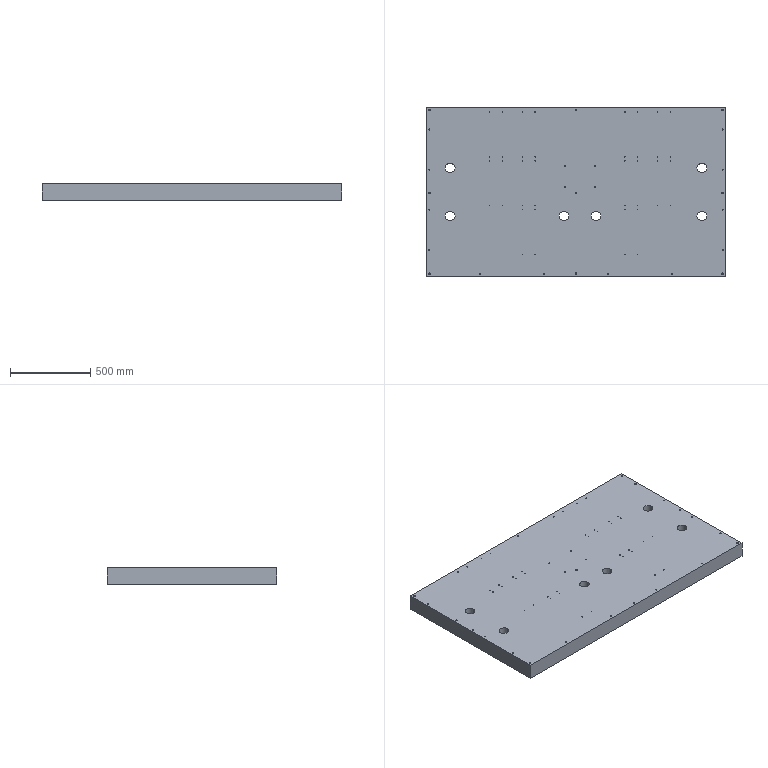Part | SolidWorks | 1 solid | 175 faces | box 1870 x 1060 x 100 mm | volume 196301866 mm3 | cylinder 160 | plane 15 | commonest cylinder face diameters 4.2 x80 6.8 x32 9 x18 15 x18 60 x12